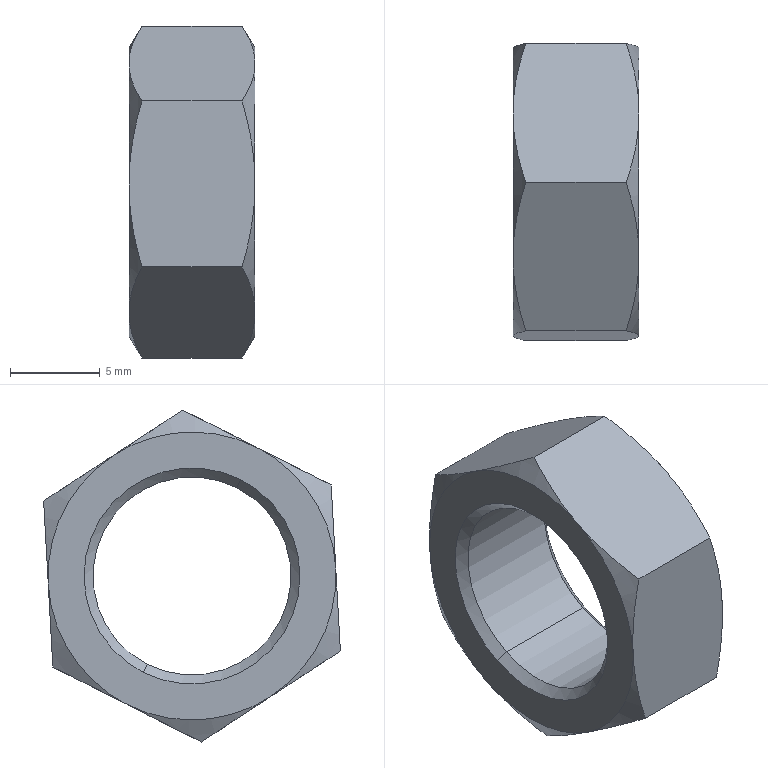Part | SolidWorks | features BaseBody 1 | 1 solid | 26 faces | box 7 x 16.489 x 18.447 mm | volume 868.886 mm3 | cone 16 | plane 8 | cylinder 2 | commonest cylinder face diameters 11 x2
STEP:
#1=CARTESIAN_POINT('',(444.6,85.519,4.909));
#2=VERTEX_POINT('',#1);
#3=CARTESIAN_POINT('',(444.6,90.481,-4.909));
#4=VERTEX_POINT('',#3);
#5=CARTESIAN_POINT('',(444.6,88.,0.));
#6=DIRECTION('',(1.,0.,0.));
#7=DIRECTION('',(0.,0.451,-0.8925));
#8=AXIS2_PLACEMENT_3D('',#5,#6,#7);
#9=CIRCLE('',#8,5.5);
#10=EDGE_CURVE('',#2,#4,#9,.T.);
#11=ORIENTED_EDGE('',*,*,#10,.F.);
#12=CARTESIAN_POINT('',(445.1,85.294,5.355));
#13=VERTEX_POINT('',#12);
#14=CARTESIAN_POINT('',(444.6,85.519,4.909));
#15=DIRECTION('',(0.7071,-0.3189,0.6311));
#16=VECTOR('',#15,1000.);
#17=LINE('',#14,#16);
#18=EDGE_CURVE('',#2,#13,#17,.T.);
#19=ORIENTED_EDGE('',*,*,#18,.T.);
#20=CARTESIAN_POINT('',(445.1,90.706,-5.355));
#21=VERTEX_POINT('',#20);
#22=CARTESIAN_POINT('',(445.1,88.,0.));
#23=DIRECTION('',(-1.,0.,0.));
#24=DIRECTION('',(0.,0.451,-0.8925));
#25=AXIS2_PLACEMENT_3D('',#22,#23,#24);
#26=CIRCLE('',#25,6.);
#27=EDGE_CURVE('',#21,#13,#26,.T.);
#28=ORIENTED_EDGE('',*,*,#27,.F.);
#29=CARTESIAN_POINT('',(444.6,90.481,-4.909));
#30=DIRECTION('',(0.7071,0.3189,-0.6311));
#31=VECTOR('',#30,1000.);
#32=LINE('',#29,#31);
#33=EDGE_CURVE('',#4,#21,#32,.T.);
#34=ORIENTED_EDGE('',*,*,#33,.F.);
#35=EDGE_LOOP('',(#11,#19,#28,#34));
#36=FACE_OUTER_BOUND('',#35,.T.);
#37=CARTESIAN_POINT('',(444.6,88.,0.));
#38=DIRECTION('',(1.,0.,0.));
#39=DIRECTION('',(0.,0.451,-0.8925));
#40=AXIS2_PLACEMENT_3D('',#37,#38,#39);
#41=CONICAL_SURFACE('',#40,5.5,0.7854);
#42=ADVANCED_FACE('',(#36),#41,.F.);
#43=CARTESIAN_POINT('',(438.6,90.481,-4.909));
#44=VERTEX_POINT('',#43);
#45=CARTESIAN_POINT('',(438.6,85.519,4.909));
#46=VERTEX_POINT('',#45);
#47=CARTESIAN_POINT('',(438.6,88.,0.));
#48=DIRECTION('',(-1.,0.,0.));
#49=DIRECTION('',(0.,0.451,-0.8925));
#50=AXIS2_PLACEMENT_3D('',#47,#48,#49);
#51=CIRCLE('',#50,5.5);
#52=EDGE_CURVE('',#44,#46,#51,.T.);
#53=ORIENTED_EDGE('',*,*,#52,.F.);
#54=CARTESIAN_POINT('',(438.1,90.706,-5.355));
#55=VERTEX_POINT('',#54);
#56=CARTESIAN_POINT('',(438.1,90.706,-5.355));
#57=DIRECTION('',(-0.7071,0.3189,-0.6311));
#58=VECTOR('',#57,1000.);
#59=LINE('',#56,#58);
#60=EDGE_CURVE('',#44,#55,#59,.T.);
#61=ORIENTED_EDGE('',*,*,#60,.T.);
#62=CARTESIAN_POINT('',(438.1,85.294,5.355));
#63=VERTEX_POINT('',#62);
#64=CARTESIAN_POINT('',(438.1,88.,0.));
#65=DIRECTION('',(1.,0.,0.));
#66=DIRECTION('',(0.,0.451,-0.8925));
#67=AXIS2_PLACEMENT_3D('',#64,#65,#66);
#68=CIRCLE('',#67,6.);
#69=EDGE_CURVE('',#63,#55,#68,.T.);
#70=ORIENTED_EDGE('',*,*,#69,.F.);
#71=CARTESIAN_POINT('',(438.1,85.294,5.355));
#72=DIRECTION('',(-0.7071,-0.3189,0.6311));
#73=VECTOR('',#72,1000.);
#74=LINE('',#71,#73);
#75=EDGE_CURVE('',#46,#63,#74,.T.);
#76=ORIENTED_EDGE('',*,*,#75,.F.);
#77=EDGE_LOOP('',(#53,#61,#70,#76));
#78=FACE_OUTER_BOUND('',#77,.T.);
#79=CARTESIAN_POINT('',(438.1,88.,0.));
#80=DIRECTION('',(-1.,0.,0.));
#81=DIRECTION('',(0.,-0.451,0.8925));
#82=AXIS2_PLACEMENT_3D('',#79,#80,#81);
#83=CONICAL_SURFACE('',#82,6.,0.7854);
#84=ADVANCED_FACE('',(#78),#83,.F.);
#85=ORIENTED_EDGE('',*,*,#52,.T.);
#86=CARTESIAN_POINT('',(438.1,85.519,4.909));
#87=DIRECTION('',(1.,0.,0.));
#88=VECTOR('',#87,1000.);
#89=LINE('',#86,#88);
#90=EDGE_CURVE('',#46,#2,#89,.T.);
#91=ORIENTED_EDGE('',*,*,#90,.T.);
#92=ORIENTED_EDGE('',*,*,#10,.T.);
#93=CARTESIAN_POINT('',(438.1,90.481,-4.909));
#94=DIRECTION('',(1.,0.,0.));
#95=VECTOR('',#94,1000.);
#96=LINE('',#93,#95);
#97=EDGE_CURVE('',#44,#4,#96,.T.);
#98=ORIENTED_EDGE('',*,*,#97,.F.);
#99=EDGE_LOOP('',(#85,#91,#92,#98));
#100=FACE_OUTER_BOUND('',#99,.T.);
#101=CARTESIAN_POINT('',(438.1,88.,0.));
#102=DIRECTION('',(1.,0.,0.));
#103=DIRECTION('',(0.,0.451,-0.8925));
#104=AXIS2_PLACEMENT_3D('',#101,#102,#103);
#105=CYLINDRICAL_SURFACE('',#104,5.5);
#106=ADVANCED_FACE('',(#100),#105,.F.);
#107=CARTESIAN_POINT('',(438.815,96.245,4.166));
#108=VERTEX_POINT('',#107);
#109=CARTESIAN_POINT('',(438.1,95.988,-0.4454));
#110=VERTEX_POINT('',#109);
#111=CARTESIAN_POINT('',(438.815,96.245,4.166));
#112=CARTESIAN_POINT('',(438.596,96.203,3.412));
#113=CARTESIAN_POINT('',(438.417,96.16,2.652));
#114=CARTESIAN_POINT('',(438.168,96.075,1.116));
#115=CARTESIAN_POINT('',(438.1,96.031,0.3403));
#116=CARTESIAN_POINT('',(438.1,95.988,-0.4454));
#117=B_SPLINE_CURVE_WITH_KNOTS('',3,(#111,#112,#113,#114,#115,#116),.UNSPECIFIED.,.F.,.F.,(4,2,4),(0.000000238,0.002337,0.004674),.UNSPECIFIED.);
#118=EDGE_CURVE('',#108,#110,#117,.T.);
#119=ORIENTED_EDGE('',*,*,#118,.F.);
#120=CARTESIAN_POINT('',(444.385,96.245,4.166));
#121=VERTEX_POINT('',#120);
#122=CARTESIAN_POINT('',(445.1,96.245,4.166));
#123=DIRECTION('',(-1.,0.,0.));
#124=VECTOR('',#123,1000.);
#125=LINE('',#122,#124);
#126=EDGE_CURVE('',#121,#108,#125,.T.);
#127=ORIENTED_EDGE('',*,*,#126,.F.);
#128=CARTESIAN_POINT('',(445.1,95.988,-0.4454));
#129=VERTEX_POINT('',#128);
#130=CARTESIAN_POINT('',(445.1,95.988,-0.4454));
#131=CARTESIAN_POINT('',(445.1,96.009,-0.054));
#132=CARTESIAN_POINT('',(445.083,96.031,0.3391));
#133=CARTESIAN_POINT('',(445.018,96.075,1.117));
#134=CARTESIAN_POINT('',(444.969,96.096,1.503));
#135=CARTESIAN_POINT('',(444.783,96.16,2.655));
#136=CARTESIAN_POINT('',(444.603,96.203,3.414));
#137=CARTESIAN_POINT('',(444.385,96.245,4.166));
#138=B_SPLINE_CURVE_WITH_KNOTS('',3,(#130,#131,#132,#133,#134,#135,#136,#137),.UNSPECIFIED.,.F.,.F.,(4,2,2,4),(0.004674,0.005838,0.007002,0.00933),.UNSPECIFIED.);
#139=EDGE_CURVE('',#129,#121,#138,.T.);
#140=ORIENTED_EDGE('',*,*,#139,.F.);
#141=CARTESIAN_POINT('',(444.385,95.73,-5.057));
#142=VERTEX_POINT('',#141);
#143=CARTESIAN_POINT('',(444.385,95.73,-5.057));
#144=CARTESIAN_POINT('',(444.604,95.773,-4.303));
#145=CARTESIAN_POINT('',(444.783,95.815,-3.543));
#146=CARTESIAN_POINT('',(445.032,95.901,-2.007));
#147=CARTESIAN_POINT('',(445.1,95.944,-1.231));
#148=CARTESIAN_POINT('',(445.1,95.988,-0.4454));
#149=B_SPLINE_CURVE_WITH_KNOTS('',3,(#143,#144,#145,#146,#147,#148),.UNSPECIFIED.,.F.,.F.,(4,2,4),(0.000000238,0.002337,0.004674),.UNSPECIFIED.);
#150=EDGE_CURVE('',#142,#129,#149,.T.);
#151=ORIENTED_EDGE('',*,*,#150,.F.);
#152=CARTESIAN_POINT('',(438.815,95.73,-5.057));
#153=VERTEX_POINT('',#152);
#154=CARTESIAN_POINT('',(445.1,95.73,-5.057));
#155=DIRECTION('',(-1.,0.,0.));
#156=VECTOR('',#155,1000.);
#157=LINE('',#154,#156);
#158=EDGE_CURVE('',#142,#153,#157,.T.);
#159=ORIENTED_EDGE('',*,*,#158,.T.);
#160=CARTESIAN_POINT('',(438.1,95.988,-0.4454));
#161=CARTESIAN_POINT('',(438.1,95.966,-0.8367));
#162=CARTESIAN_POINT('',(438.117,95.944,-1.23));
#163=CARTESIAN_POINT('',(438.182,95.9,-2.008));
#164=CARTESIAN_POINT('',(438.231,95.879,-2.394));
#165=CARTESIAN_POINT('',(438.417,95.815,-3.546));
#166=CARTESIAN_POINT('',(438.597,95.772,-4.304));
#167=CARTESIAN_POINT('',(438.815,95.73,-5.057));
#168=B_SPLINE_CURVE_WITH_KNOTS('',3,(#160,#161,#162,#163,#164,#165,#166,#167),.UNSPECIFIED.,.F.,.F.,(4,2,2,4),(0.004674,0.005838,0.007002,0.00933),.UNSPECIFIED.);
#169=EDGE_CURVE('',#110,#153,#168,.T.);
#170=ORIENTED_EDGE('',*,*,#169,.F.);
#171=EDGE_LOOP('',(#119,#127,#140,#151,#159,#170));
#172=FACE_OUTER_BOUND('',#171,.T.);
#173=CARTESIAN_POINT('',(445.1,95.73,-5.057));
#174=DIRECTION('',(0.,-0.9984,0.05567));
#175=DIRECTION('',(0.,-0.05567,-0.9984));
#176=AXIS2_PLACEMENT_3D('',#173,#174,#175);
#177=PLANE('',#176);
#178=ADVANCED_FACE('',(#172),#177,.F.);
#179=CARTESIAN_POINT('',(438.815,88.514,9.223));
#180=VERTEX_POINT('',#179);
#181=CARTESIAN_POINT('',(438.1,92.38,6.695));
#182=VERTEX_POINT('',#181);
#183=CARTESIAN_POINT('',(438.815,88.514,9.223));
#184=CARTESIAN_POINT('',(438.596,89.147,8.81));
#185=CARTESIAN_POINT('',(438.417,89.783,8.393));
#186=CARTESIAN_POINT('',(438.168,91.071,7.551));
#187=CARTESIAN_POINT('',(438.1,91.721,7.126));
#188=CARTESIAN_POINT('',(438.1,92.38,6.695));
#189=B_SPLINE_CURVE_WITH_KNOTS('',3,(#183,#184,#185,#186,#187,#188),.UNSPECIFIED.,.F.,.F.,(4,2,4),(0.000000238,0.002337,0.004674),.UNSPECIFIED.);
#190=EDGE_CURVE('',#180,#182,#189,.T.);
#191=ORIENTED_EDGE('',*,*,#190,.F.);
#192=CARTESIAN_POINT('',(444.385,88.514,9.223));
#193=VERTEX_POINT('',#192);
#194=CARTESIAN_POINT('',(445.1,88.514,9.223));
#195=DIRECTION('',(-1.,0.,0.));
#196=VECTOR('',#195,1000.);
#197=LINE('',#194,#196);
#198=EDGE_CURVE('',#193,#180,#197,.T.);
#199=ORIENTED_EDGE('',*,*,#198,.F.);
#200=CARTESIAN_POINT('',(445.1,92.38,6.695));
#201=VERTEX_POINT('',#200);
#202=CARTESIAN_POINT('',(445.1,92.38,6.695));
#203=CARTESIAN_POINT('',(445.1,92.051,6.909));
#204=CARTESIAN_POINT('',(445.083,91.722,7.125));
#205=CARTESIAN_POINT('',(445.018,91.07,7.551));
#206=CARTESIAN_POINT('',(444.969,90.746,7.763));
#207=CARTESIAN_POINT('',(444.783,89.781,8.395));
#208=CARTESIAN_POINT('',(444.603,89.145,8.811));
#209=CARTESIAN_POINT('',(444.385,88.514,9.223));
#210=B_SPLINE_CURVE_WITH_KNOTS('',3,(#202,#203,#204,#205,#206,#207,#208,#209),.UNSPECIFIED.,.F.,.F.,(4,2,2,4),(0.004674,0.005838,0.007002,0.00933),.UNSPECIFIED.);
#211=EDGE_CURVE('',#201,#193,#210,.T.);
#212=ORIENTED_EDGE('',*,*,#211,.F.);
#213=CARTESIAN_POINT('',(444.385,96.245,4.166));
#214=CARTESIAN_POINT('',(444.604,95.612,4.58));
#215=CARTESIAN_POINT('',(444.783,94.976,4.997));
#216=CARTESIAN_POINT('',(445.032,93.688,5.839));
#217=CARTESIAN_POINT('',(445.1,93.038,6.264));
#218=CARTESIAN_POINT('',(445.1,92.38,6.695));
#219=B_SPLINE_CURVE_WITH_KNOTS('',3,(#213,#214,#215,#216,#217,#218),.UNSPECIFIED.,.F.,.F.,(4,2,4),(0.000000238,0.002337,0.004674),.UNSPECIFIED.);
#220=EDGE_CURVE('',#121,#201,#219,.T.);
#221=ORIENTED_EDGE('',*,*,#220,.F.);
#222=ORIENTED_EDGE('',*,*,#126,.T.);
#223=CARTESIAN_POINT('',(438.1,92.38,6.695));
#224=CARTESIAN_POINT('',(438.1,92.708,6.48));
#225=CARTESIAN_POINT('',(438.117,93.037,6.265));
#226=CARTESIAN_POINT('',(438.182,93.689,5.838));
#227=CARTESIAN_POINT('',(438.231,94.013,5.626));
#228=CARTESIAN_POINT('',(438.417,94.978,4.995));
#229=CARTESIAN_POINT('',(438.597,95.614,4.579));
#230=CARTESIAN_POINT('',(438.815,96.245,4.166));
#231=B_SPLINE_CURVE_WITH_KNOTS('',3,(#223,#224,#225,#226,#227,#228,#229,#230),.UNSPECIFIED.,.F.,.F.,(4,2,2,4),(0.004674,0.005838,0.007002,0.00933),.UNSPECIFIED.);
#232=EDGE_CURVE('',#182,#108,#231,.T.);
#233=ORIENTED_EDGE('',*,*,#232,.F.);
#234=EDGE_LOOP('',(#191,#199,#212,#221,#222,#233));
#235=FACE_OUTER_BOUND('',#234,.T.);
#236=CARTESIAN_POINT('',(445.1,96.245,4.166));
#237=DIRECTION('',(0.,-0.5474,-0.8368));
#238=DIRECTION('',(0.,0.8368,-0.5474));
#239=AXIS2_PLACEMENT_3D('',#236,#237,#238);
#240=PLANE('',#239);
#241=ADVANCED_FACE('',(#235),#240,.F.);
#242=CARTESIAN_POINT('',(438.815,80.27,5.057));
#243=VERTEX_POINT('',#242);
#244=CARTESIAN_POINT('',(438.1,84.392,7.14));
#245=VERTEX_POINT('',#244);
#246=CARTESIAN_POINT('',(438.815,80.27,5.057));
#247=CARTESIAN_POINT('',(438.597,80.941,5.396));
#248=CARTESIAN_POINT('',(438.416,81.627,5.743));
#249=CARTESIAN_POINT('',(438.167,83.002,6.438));
#250=CARTESIAN_POINT('',(438.1,83.694,6.788));
#251=CARTESIAN_POINT('',(438.1,84.392,7.14));
#252=B_SPLINE_CURVE_WITH_KNOTS('',3,(#246,#247,#248,#249,#250,#251),.UNSPECIFIED.,.F.,.F.,(4,2,4),(0.008651,0.01099,0.01333),.UNSPECIFIED.);
#253=EDGE_CURVE('',#243,#245,#252,.T.);
#254=ORIENTED_EDGE('',*,*,#253,.F.);
#255=CARTESIAN_POINT('',(444.385,80.27,5.057));
#256=VERTEX_POINT('',#255);
#257=CARTESIAN_POINT('',(445.1,80.27,5.057));
#258=DIRECTION('',(-1.,0.,0.));
#259=VECTOR('',#258,1000.);
#260=LINE('',#257,#259);
#261=EDGE_CURVE('',#256,#243,#260,.T.);
#262=ORIENTED_EDGE('',*,*,#261,.F.);
#263=CARTESIAN_POINT('',(445.1,84.392,7.14));
#264=VERTEX_POINT('',#263);
#265=CARTESIAN_POINT('',(445.1,84.392,7.14));
#266=CARTESIAN_POINT('',(445.1,83.694,6.788));
#267=CARTESIAN_POINT('',(445.033,83.002,6.438));
#268=CARTESIAN_POINT('',(444.784,81.627,5.743));
#269=CARTESIAN_POINT('',(444.603,80.941,5.396));
#270=CARTESIAN_POINT('',(444.385,80.27,5.057));
#271=B_SPLINE_CURVE_WITH_KNOTS('',3,(#265,#266,#267,#268,#269,#270),.UNSPECIFIED.,.F.,.F.,(4,2,4),(0.02955,0.03188,0.03422),.UNSPECIFIED.);
#272=EDGE_CURVE('',#264,#256,#271,.T.);
#273=ORIENTED_EDGE('',*,*,#272,.F.);
#274=CARTESIAN_POINT('',(444.385,88.514,9.223));
#275=CARTESIAN_POINT('',(444.601,87.847,8.886));
#276=CARTESIAN_POINT('',(444.781,87.172,8.545));
#277=CARTESIAN_POINT('',(444.968,86.141,8.024));
#278=CARTESIAN_POINT('',(445.017,85.794,7.849));
#279=CARTESIAN_POINT('',(445.083,85.093,7.494));
#280=CARTESIAN_POINT('',(445.1,84.741,7.317));
#281=CARTESIAN_POINT('',(445.1,84.392,7.14));
#282=B_SPLINE_CURVE_WITH_KNOTS('',3,(#274,#275,#276,#277,#278,#279,#280,#281),.UNSPECIFIED.,.F.,.F.,(4,2,2,4),(0.02487,0.02721,0.02838,0.02955),.UNSPECIFIED.);
#283=EDGE_CURVE('',#193,#264,#282,.T.);
#284=ORIENTED_EDGE('',*,*,#283,.F.);
#285=ORIENTED_EDGE('',*,*,#198,.T.);
#286=CARTESIAN_POINT('',(438.1,84.392,7.14));
#287=CARTESIAN_POINT('',(438.1,84.741,7.317));
#288=CARTESIAN_POINT('',(438.117,85.093,7.494));
#289=CARTESIAN_POINT('',(438.183,85.794,7.849));
#290=CARTESIAN_POINT('',(438.232,86.141,8.024));
#291=CARTESIAN_POINT('',(438.419,87.172,8.545));
#292=CARTESIAN_POINT('',(438.599,87.847,8.886));
#293=CARTESIAN_POINT('',(438.815,88.514,9.223));
#294=B_SPLINE_CURVE_WITH_KNOTS('',3,(#286,#287,#288,#289,#290,#291,#292,#293),.UNSPECIFIED.,.F.,.F.,(4,2,2,4),(0.01333,0.0145,0.01567,0.01801),.UNSPECIFIED.);
#295=EDGE_CURVE('',#245,#180,#294,.T.);
#296=ORIENTED_EDGE('',*,*,#295,.F.);
#297=EDGE_LOOP('',(#254,#262,#273,#284,#285,#296));
#298=FACE_OUTER_BOUND('',#297,.T.);
#299=CARTESIAN_POINT('',(445.1,88.514,9.223));
#300=DIRECTION('',(0.,0.451,-0.8925));
#301=DIRECTION('',(0.,0.8925,0.451));
#302=AXIS2_PLACEMENT_3D('',#299,#300,#301);
#303=PLANE('',#302);
#304=ADVANCED_FACE('',(#298),#303,.F.);
#305=CARTESIAN_POINT('',(438.815,79.755,-4.166));
#306=VERTEX_POINT('',#305);
#307=CARTESIAN_POINT('',(438.1,80.012,0.4454));
#308=VERTEX_POINT('',#307);
#309=CARTESIAN_POINT('',(438.815,79.755,-4.166));
#310=CARTESIAN_POINT('',(438.596,79.797,-3.412));
#311=CARTESIAN_POINT('',(438.417,79.84,-2.652));
#312=CARTESIAN_POINT('',(438.168,79.925,-1.116));
#313=CARTESIAN_POINT('',(438.1,79.969,-0.3403));
#314=CARTESIAN_POINT('',(438.1,80.012,0.4454));
#315=B_SPLINE_CURVE_WITH_KNOTS('',3,(#309,#310,#311,#312,#313,#314),.UNSPECIFIED.,.F.,.F.,(4,2,4),(0.000000238,0.002337,0.004674),.UNSPECIFIED.);
#316=EDGE_CURVE('',#306,#308,#315,.T.);
#317=ORIENTED_EDGE('',*,*,#316,.F.);
#318=CARTESIAN_POINT('',(444.385,79.755,-4.166));
#319=VERTEX_POINT('',#318);
#320=CARTESIAN_POINT('',(445.1,79.755,-4.166));
#321=DIRECTION('',(-1.,0.,0.));
#322=VECTOR('',#321,1000.);
#323=LINE('',#320,#322);
#324=EDGE_CURVE('',#319,#306,#323,.T.);
#325=ORIENTED_EDGE('',*,*,#324,.F.);
#326=CARTESIAN_POINT('',(445.1,80.012,0.4454));
#327=VERTEX_POINT('',#326);
#328=CARTESIAN_POINT('',(445.1,80.012,0.4454));
#329=CARTESIAN_POINT('',(445.1,79.991,0.054));
#330=CARTESIAN_POINT('',(445.083,79.969,-0.3391));
#331=CARTESIAN_POINT('',(445.018,79.925,-1.117));
#332=CARTESIAN_POINT('',(444.969,79.904,-1.503));
#333=CARTESIAN_POINT('',(444.783,79.84,-2.655));
#334=CARTESIAN_POINT('',(444.603,79.797,-3.414));
#335=CARTESIAN_POINT('',(444.385,79.755,-4.166));
#336=B_SPLINE_CURVE_WITH_KNOTS('',3,(#328,#329,#330,#331,#332,#333,#334,#335),.UNSPECIFIED.,.F.,.F.,(4,2,2,4),(0.004674,0.005838,0.007002,0.00933),.UNSPECIFIED.);
#337=EDGE_CURVE('',#327,#319,#336,.T.);
#338=ORIENTED_EDGE('',*,*,#337,.F.);
#339=CARTESIAN_POINT('',(444.385,80.27,5.057));
#340=CARTESIAN_POINT('',(444.604,80.227,4.303));
#341=CARTESIAN_POINT('',(444.783,80.185,3.543));
#342=CARTESIAN_POINT('',(445.032,80.099,2.007));
#343=CARTESIAN_POINT('',(445.1,80.056,1.231));
#344=CARTESIAN_POINT('',(445.1,80.012,0.4454));
#345=B_SPLINE_CURVE_WITH_KNOTS('',3,(#339,#340,#341,#342,#343,#344),.UNSPECIFIED.,.F.,.F.,(4,2,4),(0.000000238,0.002337,0.004674),.UNSPECIFIED.);
#346=EDGE_CURVE('',#256,#327,#345,.T.);
#347=ORIENTED_EDGE('',*,*,#346,.F.);
#348=ORIENTED_EDGE('',*,*,#261,.T.);
#349=CARTESIAN_POINT('',(438.1,80.012,0.4454));
#350=CARTESIAN_POINT('',(438.1,80.034,0.8367));
#351=CARTESIAN_POINT('',(438.117,80.056,1.23));
#352=CARTESIAN_POINT('',(438.182,80.1,2.008));
#353=CARTESIAN_POINT('',(438.231,80.121,2.394));
#354=CARTESIAN_POINT('',(438.417,80.185,3.546));
#355=CARTESIAN_POINT('',(438.597,80.228,4.304));
#356=CARTESIAN_POINT('',(438.815,80.27,5.057));
#357=B_SPLINE_CURVE_WITH_KNOTS('',3,(#349,#350,#351,#352,#353,#354,#355,#356),.UNSPECIFIED.,.F.,.F.,(4,2,2,4),(0.004674,0.005838,0.007002,0.00933),.UNSPECIFIED.);
#358=EDGE_CURVE('',#308,#243,#357,.T.);
#359=ORIENTED_EDGE('',*,*,#358,.F.);
#360=EDGE_LOOP('',(#317,#325,#338,#347,#348,#359));
#361=FACE_OUTER_BOUND('',#360,.T.);
#362=CARTESIAN_POINT('',(445.1,80.27,5.057));
#363=DIRECTION('',(0.,0.9984,-0.05567));
#364=DIRECTION('',(0.,0.05567,0.9984));
#365=AXIS2_PLACEMENT_3D('',#362,#363,#364);
#366=PLANE('',#365);
#367=ADVANCED_FACE('',(#361),#366,.F.);
#368=CARTESIAN_POINT('',(438.815,87.486,-9.223));
#369=VERTEX_POINT('',#368);
#370=CARTESIAN_POINT('',(438.1,83.62,-6.695));
#371=VERTEX_POINT('',#370);
#372=CARTESIAN_POINT('',(438.815,87.486,-9.223));
#373=CARTESIAN_POINT('',(438.596,86.853,-8.81));
#374=CARTESIAN_POINT('',(438.417,86.217,-8.393));
#375=CARTESIAN_POINT('',(438.168,84.929,-7.551));
#376=CARTESIAN_POINT('',(438.1,84.279,-7.126));
#377=CARTESIAN_POINT('',(438.1,83.62,-6.695));
#378=B_SPLINE_CURVE_WITH_KNOTS('',3,(#372,#373,#374,#375,#376,#377),.UNSPECIFIED.,.F.,.F.,(4,2,4),(0.000000238,0.002337,0.004674),.UNSPECIFIED.);
#379=EDGE_CURVE('',#369,#371,#378,.T.);
#380=ORIENTED_EDGE('',*,*,#379,.F.);
#381=CARTESIAN_POINT('',(444.385,87.486,-9.223));
#382=VERTEX_POINT('',#381);
#383=CARTESIAN_POINT('',(445.1,87.486,-9.223));
#384=DIRECTION('',(-1.,0.,0.));
#385=VECTOR('',#384,1000.);
#386=LINE('',#383,#385);
#387=EDGE_CURVE('',#382,#369,#386,.T.);
#388=ORIENTED_EDGE('',*,*,#387,.F.);
#389=CARTESIAN_POINT('',(445.1,83.62,-6.695));
#390=VERTEX_POINT('',#389);
#391=CARTESIAN_POINT('',(445.1,83.62,-6.695));
#392=CARTESIAN_POINT('',(445.1,83.949,-6.909));
#393=CARTESIAN_POINT('',(445.083,84.278,-7.125));
#394=CARTESIAN_POINT('',(445.018,84.93,-7.551));
#395=CARTESIAN_POINT('',(444.969,85.254,-7.763));
#396=CARTESIAN_POINT('',(444.783,86.219,-8.395));
#397=CARTESIAN_POINT('',(444.603,86.855,-8.811));
#398=CARTESIAN_POINT('',(444.385,87.486,-9.223));
#399=B_SPLINE_CURVE_WITH_KNOTS('',3,(#391,#392,#393,#394,#395,#396,#397,#398),.UNSPECIFIED.,.F.,.F.,(4,2,2,4),(0.004674,0.005838,0.007002,0.00933),.UNSPECIFIED.);
#400=EDGE_CURVE('',#390,#382,#399,.T.);
#401=ORIENTED_EDGE('',*,*,#400,.F.);
#402=CARTESIAN_POINT('',(444.385,79.755,-4.166));
#403=CARTESIAN_POINT('',(444.604,80.388,-4.58));
#404=CARTESIAN_POINT('',(444.783,81.024,-4.997));
#405=CARTESIAN_POINT('',(445.032,82.312,-5.839));
#406=CARTESIAN_POINT('',(445.1,82.962,-6.264));
#407=CARTESIAN_POINT('',(445.1,83.62,-6.695));
#408=B_SPLINE_CURVE_WITH_KNOTS('',3,(#402,#403,#404,#405,#406,#407),.UNSPECIFIED.,.F.,.F.,(4,2,4),(0.000000238,0.002337,0.004674),.UNSPECIFIED.);
#409=EDGE_CURVE('',#319,#390,#408,.T.);
#410=ORIENTED_EDGE('',*,*,#409,.F.);
#411=ORIENTED_EDGE('',*,*,#324,.T.);
#412=CARTESIAN_POINT('',(438.1,83.62,-6.695));
#413=CARTESIAN_POINT('',(438.1,83.292,-6.48));
#414=CARTESIAN_POINT('',(438.117,82.963,-6.265));
#415=CARTESIAN_POINT('',(438.182,82.311,-5.838));
#416=CARTESIAN_POINT('',(438.231,81.987,-5.626));
#417=CARTESIAN_POINT('',(438.417,81.022,-4.995));
#418=CARTESIAN_POINT('',(438.597,80.386,-4.579));
#419=CARTESIAN_POINT('',(438.815,79.755,-4.166));
#420=B_SPLINE_CURVE_WITH_KNOTS('',3,(#412,#413,#414,#415,#416,#417,#418,#419),.UNSPECIFIED.,.F.,.F.,(4,2,2,4),(0.004674,0.005838,0.007002,0.00933),.UNSPECIFIED.);
#421=EDGE_CURVE('',#371,#306,#420,.T.);
#422=ORIENTED_EDGE('',*,*,#421,.F.);
#423=EDGE_LOOP('',(#380,#388,#401,#410,#411,#422));
#424=FACE_OUTER_BOUND('',#423,.T.);
#425=CARTESIAN_POINT('',(445.1,79.755,-4.166));
#426=DIRECTION('',(0.,0.5474,0.8368));
#427=DIRECTION('',(0.,-0.8368,0.5474));
#428=AXIS2_PLACEMENT_3D('',#425,#426,#427);
#429=PLANE('',#428);
#430=ADVANCED_FACE('',(#424),#429,.F.);
#431=CARTESIAN_POINT('',(438.1,91.608,-7.14));
#432=VERTEX_POINT('',#431);
#433=CARTESIAN_POINT('',(438.815,95.73,-5.057));
#434=CARTESIAN_POINT('',(438.599,95.064,-5.394));
#435=CARTESIAN_POINT('',(438.419,94.388,-5.735));
#436=CARTESIAN_POINT('',(438.232,93.357,-6.256));
#437=CARTESIAN_POINT('',(438.183,93.01,-6.432));
#438=CARTESIAN_POINT('',(438.117,92.309,-6.786));
#439=CARTESIAN_POINT('',(438.1,91.957,-6.964));
#440=CARTESIAN_POINT('',(438.1,91.608,-7.14));
#441=B_SPLINE_CURVE_WITH_KNOTS('',3,(#433,#434,#435,#436,#437,#438,#439,#440),.UNSPECIFIED.,.F.,.F.,(4,2,2,4),(0.02487,0.02721,0.02838,0.02955),.UNSPECIFIED.);
#442=EDGE_CURVE('',#153,#432,#441,.T.);
#443=ORIENTED_EDGE('',*,*,#442,.F.);
#444=ORIENTED_EDGE('',*,*,#158,.F.);
#445=CARTESIAN_POINT('',(445.1,91.608,-7.14));
#446=VERTEX_POINT('',#445);
#447=CARTESIAN_POINT('',(445.1,91.608,-7.14));
#448=CARTESIAN_POINT('',(445.1,91.957,-6.964));
#449=CARTESIAN_POINT('',(445.083,92.309,-6.786));
#450=CARTESIAN_POINT('',(445.017,93.01,-6.432));
#451=CARTESIAN_POINT('',(444.968,93.357,-6.256));
#452=CARTESIAN_POINT('',(444.781,94.388,-5.735));
#453=CARTESIAN_POINT('',(444.601,95.064,-5.394));
#454=CARTESIAN_POINT('',(444.385,95.73,-5.057));
#455=B_SPLINE_CURVE_WITH_KNOTS('',3,(#447,#448,#449,#450,#451,#452,#453,#454),.UNSPECIFIED.,.F.,.F.,(4,2,2,4),(0.01333,0.0145,0.01567,0.01801),.UNSPECIFIED.);
#456=EDGE_CURVE('',#446,#142,#455,.T.);
#457=ORIENTED_EDGE('',*,*,#456,.F.);
#458=CARTESIAN_POINT('',(444.385,87.486,-9.223));
#459=CARTESIAN_POINT('',(444.603,88.157,-8.884));
#460=CARTESIAN_POINT('',(444.784,88.843,-8.537));
#461=CARTESIAN_POINT('',(445.033,90.218,-7.843));
#462=CARTESIAN_POINT('',(445.1,90.91,-7.493));
#463=CARTESIAN_POINT('',(445.1,91.608,-7.14));
#464=B_SPLINE_CURVE_WITH_KNOTS('',3,(#458,#459,#460,#461,#462,#463),.UNSPECIFIED.,.F.,.F.,(4,2,4),(0.008651,0.01099,0.01333),.UNSPECIFIED.);
#465=EDGE_CURVE('',#382,#446,#464,.T.);
#466=ORIENTED_EDGE('',*,*,#465,.F.);
#467=ORIENTED_EDGE('',*,*,#387,.T.);
#468=CARTESIAN_POINT('',(438.1,91.608,-7.14));
#469=CARTESIAN_POINT('',(438.1,90.91,-7.493));
#470=CARTESIAN_POINT('',(438.167,90.218,-7.843));
#471=CARTESIAN_POINT('',(438.416,88.843,-8.537));
#472=CARTESIAN_POINT('',(438.597,88.157,-8.884));
#473=CARTESIAN_POINT('',(438.815,87.486,-9.223));
#474=B_SPLINE_CURVE_WITH_KNOTS('',3,(#468,#469,#470,#471,#472,#473),.UNSPECIFIED.,.F.,.F.,(4,2,4),(0.02955,0.03188,0.03422),.UNSPECIFIED.);
#475=EDGE_CURVE('',#432,#369,#474,.T.);
#476=ORIENTED_EDGE('',*,*,#475,.F.);
#477=EDGE_LOOP('',(#443,#444,#457,#466,#467,#476));
#478=FACE_OUTER_BOUND('',#477,.T.);
#479=CARTESIAN_POINT('',(445.1,87.486,-9.223));
#480=DIRECTION('',(0.,-0.451,0.8925));
#481=DIRECTION('',(0.,-0.8925,-0.451));
#482=AXIS2_PLACEMENT_3D('',#479,#480,#481);
#483=PLANE('',#482);
#484=ADVANCED_FACE('',(#478),#483,.F.);
#485=ORIENTED_EDGE('',*,*,#400,.T.);
#486=ORIENTED_EDGE('',*,*,#465,.T.);
#487=CARTESIAN_POINT('',(445.1,88.,0.));
#488=DIRECTION('',(1.,0.,0.));
#489=DIRECTION('',(0.,0.451,-0.8925));
#490=AXIS2_PLACEMENT_3D('',#487,#488,#489);
#491=CIRCLE('',#490,8.);
#492=EDGE_CURVE('',#390,#446,#491,.T.);
#493=ORIENTED_EDGE('',*,*,#492,.F.);
#494=EDGE_LOOP('',(#485,#486,#493));
#495=FACE_OUTER_BOUND('',#494,.T.);
#496=CARTESIAN_POINT('',(445.1,88.,0.));
#497=DIRECTION('',(-1.,0.,0.));
#498=DIRECTION('',(0.,0.451,-0.8925));
#499=AXIS2_PLACEMENT_3D('',#496,#497,#498);
#500=CONICAL_SURFACE('',#499,8.,1.047);
#501=ADVANCED_FACE('',(#495),#500,.T.);
#502=ORIENTED_EDGE('',*,*,#337,.T.);
#503=ORIENTED_EDGE('',*,*,#409,.T.);
#504=CARTESIAN_POINT('',(445.1,88.,0.));
#505=DIRECTION('',(1.,0.,0.));
#506=DIRECTION('',(0.,0.451,-0.8925));
#507=AXIS2_PLACEMENT_3D('',#504,#505,#506);
#508=CIRCLE('',#507,8.);
#509=EDGE_CURVE('',#327,#390,#508,.T.);
#510=ORIENTED_EDGE('',*,*,#509,.F.);
#511=EDGE_LOOP('',(#502,#503,#510));
#512=FACE_OUTER_BOUND('',#511,.T.);
#513=CARTESIAN_POINT('',(445.1,88.,0.));
#514=DIRECTION('',(-1.,0.,0.));
#515=DIRECTION('',(0.,0.451,-0.8925));
#516=AXIS2_PLACEMENT_3D('',#513,#514,#515);
#517=CONICAL_SURFACE('',#516,8.,1.047);
#518=ADVANCED_FACE('',(#512),#517,.T.);
#519=ORIENTED_EDGE('',*,*,#272,.T.);
#520=ORIENTED_EDGE('',*,*,#346,.T.);
#521=CARTESIAN_POINT('',(445.1,88.,0.));
#522=DIRECTION('',(1.,0.,0.));
#523=DIRECTION('',(0.,0.451,-0.8925));
#524=AXIS2_PLACEMENT_3D('',#521,#522,#523);
#525=CIRCLE('',#524,8.);
#526=EDGE_CURVE('',#264,#327,#525,.T.);
#527=ORIENTED_EDGE('',*,*,#526,.F.);
#528=EDGE_LOOP('',(#519,#520,#527));
#529=FACE_OUTER_BOUND('',#528,.T.);
#530=CARTESIAN_POINT('',(445.1,88.,0.));
#531=DIRECTION('',(-1.,0.,0.));
#532=DIRECTION('',(0.,0.451,-0.8925));
#533=AXIS2_PLACEMENT_3D('',#530,#531,#532);
#534=CONICAL_SURFACE('',#533,8.,1.047);
#535=ADVANCED_FACE('',(#529),#534,.T.);
#536=ORIENTED_EDGE('',*,*,#211,.T.);
#537=ORIENTED_EDGE('',*,*,#283,.T.);
#538=CARTESIAN_POINT('',(445.1,88.,0.));
#539=DIRECTION('',(1.,0.,0.));
#540=DIRECTION('',(0.,0.451,-0.8925));
#541=AXIS2_PLACEMENT_3D('',#538,#539,#540);
#542=CIRCLE('',#541,8.);
#543=EDGE_CURVE('',#201,#264,#542,.T.);
#544=ORIENTED_EDGE('',*,*,#543,.F.);
#545=EDGE_LOOP('',(#536,#537,#544));
#546=FACE_OUTER_BOUND('',#545,.T.);
#547=CARTESIAN_POINT('',(445.1,88.,0.));
#548=DIRECTION('',(-1.,0.,0.));
#549=DIRECTION('',(0.,0.451,-0.8925));
#550=AXIS2_PLACEMENT_3D('',#547,#548,#549);
#551=CONICAL_SURFACE('',#550,8.,1.047);
#552=ADVANCED_FACE('',(#546),#551,.T.);
#553=ORIENTED_EDGE('',*,*,#139,.T.);
#554=ORIENTED_EDGE('',*,*,#220,.T.);
#555=CARTESIAN_POINT('',(445.1,88.,0.));
#556=DIRECTION('',(1.,0.,0.));
#557=DIRECTION('',(0.,0.451,-0.8925));
#558=AXIS2_PLACEMENT_3D('',#555,#556,#557);
#559=CIRCLE('',#558,8.);
#560=EDGE_CURVE('',#129,#201,#559,.T.);
#561=ORIENTED_EDGE('',*,*,#560,.F.);
#562=EDGE_LOOP('',(#553,#554,#561));
#563=FACE_OUTER_BOUND('',#562,.T.);
#564=CARTESIAN_POINT('',(445.1,88.,0.));
#565=DIRECTION('',(-1.,0.,0.));
#566=DIRECTION('',(0.,0.451,-0.8925));
#567=AXIS2_PLACEMENT_3D('',#564,#565,#566);
#568=CONICAL_SURFACE('',#567,8.,1.047);
#569=ADVANCED_FACE('',(#563),#568,.T.);
#570=ORIENTED_EDGE('',*,*,#150,.T.);
#571=CARTESIAN_POINT('',(445.1,88.,0.));
#572=DIRECTION('',(1.,0.,0.));
#573=DIRECTION('',(0.,0.451,-0.8925));
#574=AXIS2_PLACEMENT_3D('',#571,#572,#573);
#575=CIRCLE('',#574,8.);
#576=EDGE_CURVE('',#446,#129,#575,.T.);
#577=ORIENTED_EDGE('',*,*,#576,.F.);
#578=ORIENTED_EDGE('',*,*,#456,.T.);
#579=EDGE_LOOP('',(#570,#577,#578));
#580=FACE_OUTER_BOUND('',#579,.T.);
#581=CARTESIAN_POINT('',(445.1,88.,0.));
#582=DIRECTION('',(-1.,0.,0.));
#583=DIRECTION('',(0.,0.451,-0.8925));
#584=AXIS2_PLACEMENT_3D('',#581,#582,#583);
#585=CONICAL_SURFACE('',#584,8.,1.047);
#586=ADVANCED_FACE('',(#580),#585,.T.);
#587=ORIENTED_EDGE('',*,*,#27,.T.);
#588=CARTESIAN_POINT('',(445.1,88.,0.));
#589=DIRECTION('',(-1.,0.,0.));
#590=DIRECTION('',(0.,0.451,-0.8925));
#591=AXIS2_PLACEMENT_3D('',#588,#589,#590);
#592=CIRCLE('',#591,6.);
#593=EDGE_CURVE('',#13,#21,#592,.T.);
#594=ORIENTED_EDGE('',*,*,#593,.T.);
#595=EDGE_LOOP('',(#587,#594));
#596=FACE_BOUND('',#595,.T.);
#597=ORIENTED_EDGE('',*,*,#492,.T.);
#598=ORIENTED_EDGE('',*,*,#576,.T.);
#599=ORIENTED_EDGE('',*,*,#560,.T.);
#600=ORIENTED_EDGE('',*,*,#543,.T.);
#601=ORIENTED_EDGE('',*,*,#526,.T.);
#602=ORIENTED_EDGE('',*,*,#509,.T.);
#603=EDGE_LOOP('',(#597,#598,#599,#600,#601,#602));
#604=FACE_OUTER_BOUND('',#603,.T.);
#605=CARTESIAN_POINT('',(445.1,96.759,13.39));
#606=DIRECTION('',(1.,0.,0.));
#607=DIRECTION('',(0.,0.451,-0.8925));
#608=AXIS2_PLACEMENT_3D('',#605,#606,#607);
#609=PLANE('',#608);
#610=ADVANCED_FACE('',(#596,#604),#609,.T.);
#611=ORIENTED_EDGE('',*,*,#379,.T.);
#612=CARTESIAN_POINT('',(438.1,88.,0.));
#613=DIRECTION('',(1.,0.,0.));
#614=DIRECTION('',(0.,0.451,-0.8925));
#615=AXIS2_PLACEMENT_3D('',#612,#613,#614);
#616=CIRCLE('',#615,8.);
#617=EDGE_CURVE('',#371,#432,#616,.T.);
#618=ORIENTED_EDGE('',*,*,#617,.T.);
#619=ORIENTED_EDGE('',*,*,#475,.T.);
#620=EDGE_LOOP('',(#611,#618,#619));
#621=FACE_OUTER_BOUND('',#620,.T.);
#622=CARTESIAN_POINT('',(438.1,88.,0.));
#623=DIRECTION('',(1.,0.,0.));
#624=DIRECTION('',(0.,-0.451,0.8925));
#625=AXIS2_PLACEMENT_3D('',#622,#623,#624);
#626=CONICAL_SURFACE('',#625,8.,1.047);
#627=ADVANCED_FACE('',(#621),#626,.T.);
#628=ORIENTED_EDGE('',*,*,#316,.T.);
#629=CARTESIAN_POINT('',(438.1,88.,0.));
#630=DIRECTION('',(1.,0.,0.));
#631=DIRECTION('',(0.,0.451,-0.8925));
#632=AXIS2_PLACEMENT_3D('',#629,#630,#631);
#633=CIRCLE('',#632,8.);
#634=EDGE_CURVE('',#308,#371,#633,.T.);
#635=ORIENTED_EDGE('',*,*,#634,.T.);
#636=ORIENTED_EDGE('',*,*,#421,.T.);
#637=EDGE_LOOP('',(#628,#635,#636));
#638=FACE_OUTER_BOUND('',#637,.T.);
#639=CARTESIAN_POINT('',(438.1,88.,0.));
#640=DIRECTION('',(1.,0.,0.));
#641=DIRECTION('',(0.,-0.451,0.8925));
#642=AXIS2_PLACEMENT_3D('',#639,#640,#641);
#643=CONICAL_SURFACE('',#642,8.,1.047);
#644=ADVANCED_FACE('',(#638),#643,.T.);
#645=ORIENTED_EDGE('',*,*,#253,.T.);
#646=CARTESIAN_POINT('',(438.1,88.,0.));
#647=DIRECTION('',(1.,0.,0.));
#648=DIRECTION('',(0.,0.451,-0.8925));
#649=AXIS2_PLACEMENT_3D('',#646,#647,#648);
#650=CIRCLE('',#649,8.);
#651=EDGE_CURVE('',#245,#308,#650,.T.);
#652=ORIENTED_EDGE('',*,*,#651,.T.);
#653=ORIENTED_EDGE('',*,*,#358,.T.);
#654=EDGE_LOOP('',(#645,#652,#653));
#655=FACE_OUTER_BOUND('',#654,.T.);
#656=CARTESIAN_POINT('',(438.1,88.,0.));
#657=DIRECTION('',(1.,0.,0.));
#658=DIRECTION('',(0.,-0.451,0.8925));
#659=AXIS2_PLACEMENT_3D('',#656,#657,#658);
#660=CONICAL_SURFACE('',#659,8.,1.047);
#661=ADVANCED_FACE('',(#655),#660,.T.);
#662=ORIENTED_EDGE('',*,*,#295,.T.);
#663=ORIENTED_EDGE('',*,*,#190,.T.);
#664=CARTESIAN_POINT('',(438.1,88.,0.));
#665=DIRECTION('',(-1.,0.,0.));
#666=DIRECTION('',(0.,-0.451,0.8925));
#667=AXIS2_PLACEMENT_3D('',#664,#665,#666);
#668=CIRCLE('',#667,8.);
#669=EDGE_CURVE('',#245,#182,#668,.T.);
#670=ORIENTED_EDGE('',*,*,#669,.F.);
#671=EDGE_LOOP('',(#662,#663,#670));
#672=FACE_OUTER_BOUND('',#671,.T.);
#673=CARTESIAN_POINT('',(438.1,88.,0.));
#674=DIRECTION('',(1.,0.,0.));
#675=DIRECTION('',(0.,-0.451,0.8925));
#676=AXIS2_PLACEMENT_3D('',#673,#674,#675);
#677=CONICAL_SURFACE('',#676,8.,1.047);
#678=ADVANCED_FACE('',(#672),#677,.T.);
#679=ORIENTED_EDGE('',*,*,#232,.T.);
#680=ORIENTED_EDGE('',*,*,#118,.T.);
#681=CARTESIAN_POINT('',(438.1,88.,0.));
#682=DIRECTION('',(1.,0.,0.));
#683=DIRECTION('',(0.,0.451,-0.8925));
#684=AXIS2_PLACEMENT_3D('',#681,#682,#683);
#685=CIRCLE('',#684,8.);
#686=EDGE_CURVE('',#110,#182,#685,.T.);
#687=ORIENTED_EDGE('',*,*,#686,.T.);
#688=EDGE_LOOP('',(#679,#680,#687));
#689=FACE_OUTER_BOUND('',#688,.T.);
#690=CARTESIAN_POINT('',(438.1,88.,0.));
#691=DIRECTION('',(1.,0.,0.));
#692=DIRECTION('',(0.,-0.451,0.8925));
#693=AXIS2_PLACEMENT_3D('',#690,#691,#692);
#694=CONICAL_SURFACE('',#693,8.,1.047);
#695=ADVANCED_FACE('',(#689),#694,.T.);
#696=ORIENTED_EDGE('',*,*,#169,.T.);
#697=ORIENTED_EDGE('',*,*,#442,.T.);
#698=CARTESIAN_POINT('',(438.1,88.,0.));
#699=DIRECTION('',(1.,0.,0.));
#700=DIRECTION('',(0.,0.451,-0.8925));
#701=AXIS2_PLACEMENT_3D('',#698,#699,#700);
#702=CIRCLE('',#701,8.);
#703=EDGE_CURVE('',#432,#110,#702,.T.);
#704=ORIENTED_EDGE('',*,*,#703,.T.);
#705=EDGE_LOOP('',(#696,#697,#704));
#706=FACE_OUTER_BOUND('',#705,.T.);
#707=CARTESIAN_POINT('',(438.1,88.,0.));
#708=DIRECTION('',(1.,0.,0.));
#709=DIRECTION('',(0.,-0.451,0.8925));
#710=AXIS2_PLACEMENT_3D('',#707,#708,#709);
#711=CONICAL_SURFACE('',#710,8.,1.047);
#712=ADVANCED_FACE('',(#706),#711,.T.);
#713=ORIENTED_EDGE('',*,*,#69,.T.);
#714=CARTESIAN_POINT('',(438.1,88.,0.));
#715=DIRECTION('',(1.,0.,0.));
#716=DIRECTION('',(0.,0.451,-0.8925));
#717=AXIS2_PLACEMENT_3D('',#714,#715,#716);
#718=CIRCLE('',#717,6.);
#719=EDGE_CURVE('',#55,#63,#718,.T.);
#720=ORIENTED_EDGE('',*,*,#719,.T.);
#721=EDGE_LOOP('',(#713,#720));
#722=FACE_BOUND('',#721,.T.);
#723=ORIENTED_EDGE('',*,*,#703,.F.);
#724=ORIENTED_EDGE('',*,*,#617,.F.);
#725=ORIENTED_EDGE('',*,*,#634,.F.);
#726=ORIENTED_EDGE('',*,*,#651,.F.);
#727=ORIENTED_EDGE('',*,*,#669,.T.);
#728=ORIENTED_EDGE('',*,*,#686,.F.);
#729=EDGE_LOOP('',(#723,#724,#725,#726,#727,#728));
#730=FACE_OUTER_BOUND('',#729,.T.);
#731=CARTESIAN_POINT('',(438.1,96.759,13.39));
#732=DIRECTION('',(1.,0.,0.));
#733=DIRECTION('',(0.,0.451,-0.8925));
#734=AXIS2_PLACEMENT_3D('',#731,#732,#733);
#735=PLANE('',#734);
#736=ADVANCED_FACE('',(#722,#730),#735,.F.);
#737=ORIENTED_EDGE('',*,*,#90,.F.);
#738=CARTESIAN_POINT('',(438.6,88.,0.));
#739=DIRECTION('',(-1.,0.,0.));
#740=DIRECTION('',(0.,0.451,-0.8925));
#741=AXIS2_PLACEMENT_3D('',#738,#739,#740);
#742=CIRCLE('',#741,5.5);
#743=EDGE_CURVE('',#46,#44,#742,.T.);
#744=ORIENTED_EDGE('',*,*,#743,.T.);
#745=ORIENTED_EDGE('',*,*,#97,.T.);
#746=CARTESIAN_POINT('',(444.6,88.,0.));
#747=DIRECTION('',(1.,0.,0.));
#748=DIRECTION('',(0.,0.451,-0.8925));
#749=AXIS2_PLACEMENT_3D('',#746,#747,#748);
#750=CIRCLE('',#749,5.5);
#751=EDGE_CURVE('',#4,#2,#750,.T.);
#752=ORIENTED_EDGE('',*,*,#751,.T.);
#753=EDGE_LOOP('',(#737,#744,#745,#752));
#754=FACE_OUTER_BOUND('',#753,.T.);
#755=CARTESIAN_POINT('',(438.1,88.,0.));
#756=DIRECTION('',(1.,0.,0.));
#757=DIRECTION('',(0.,0.451,-0.8925));
#758=AXIS2_PLACEMENT_3D('',#755,#756,#757);
#759=CYLINDRICAL_SURFACE('',#758,5.5);
#760=ADVANCED_FACE('',(#754),#759,.F.);
#761=ORIENTED_EDGE('',*,*,#60,.F.);
#762=ORIENTED_EDGE('',*,*,#743,.F.);
#763=ORIENTED_EDGE('',*,*,#75,.T.);
#764=ORIENTED_EDGE('',*,*,#719,.F.);
#765=EDGE_LOOP('',(#761,#762,#763,#764));
#766=FACE_OUTER_BOUND('',#765,.T.);
#767=CARTESIAN_POINT('',(438.1,88.,0.));
#768=DIRECTION('',(-1.,0.,0.));
#769=DIRECTION('',(0.,-0.451,0.8925));
#770=AXIS2_PLACEMENT_3D('',#767,#768,#769);
#771=CONICAL_SURFACE('',#770,6.,0.7854);
#772=ADVANCED_FACE('',(#766),#771,.F.);
#773=ORIENTED_EDGE('',*,*,#18,.F.);
#774=ORIENTED_EDGE('',*,*,#751,.F.);
#775=ORIENTED_EDGE('',*,*,#33,.T.);
#776=ORIENTED_EDGE('',*,*,#593,.F.);
#777=EDGE_LOOP('',(#773,#774,#775,#776));
#778=FACE_OUTER_BOUND('',#777,.T.);
#779=CARTESIAN_POINT('',(444.6,88.,0.));
#780=DIRECTION('',(1.,0.,0.));
#781=DIRECTION('',(0.,0.451,-0.8925));
#782=AXIS2_PLACEMENT_3D('',#779,#780,#781);
#783=CONICAL_SURFACE('',#782,5.5,0.7854);
#784=ADVANCED_FACE('',(#778),#783,.F.);
#785=CLOSED_SHELL('',(#42,#84,#106,#178,#241,#304,#367,#430,#484,#501,#518,#535,#552,#569,#586,#610,#627,#644,#661,#678,#695,#712,#736,#760,#772,#784));
#786=MANIFOLD_SOLID_BREP('',#785);
#787=CARTESIAN_POINT('',(0.,0.,0.));
#788=DIRECTION('',(0.,0.,1.));
#789=DIRECTION('',(1.,0.,0.));
#790=AXIS2_PLACEMENT_3D('',#787,#788,#789);
#791=(LENGTH_UNIT()NAMED_UNIT(*)SI_UNIT(.MILLI.,.METRE.));
#792=UNCERTAINTY_MEASURE_WITH_UNIT(LENGTH_MEASURE(0.00001),#791,'','');
#793=(NAMED_UNIT(*)PLANE_ANGLE_UNIT()SI_UNIT($,.RADIAN.));
#794=(NAMED_UNIT(*)SI_UNIT($,.STERADIAN.)SOLID_ANGLE_UNIT());
#795=(GEOMETRIC_REPRESENTATION_CONTEXT(3)GLOBAL_UNCERTAINTY_ASSIGNED_CONTEXT((#792))GLOBAL_UNIT_ASSIGNED_CONTEXT((#791,#793,#794))REPRESENTATION_CONTEXT('',''));
#796=ADVANCED_BREP_SHAPE_REPRESENTATION('',(#786,#790),#795);